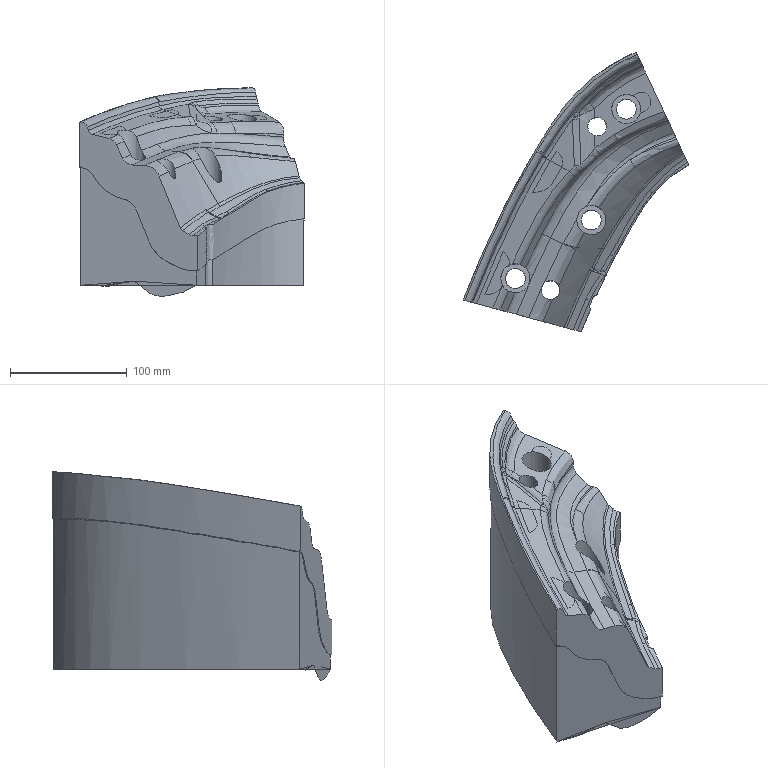Part | NX | features solid 2 | 1 solid | 107 faces | volume 2473221 mm3 | spline 88 | cylinder 10 | plane 9 | commonest cylinder face diameters 25 x5 17 x3 16 x2